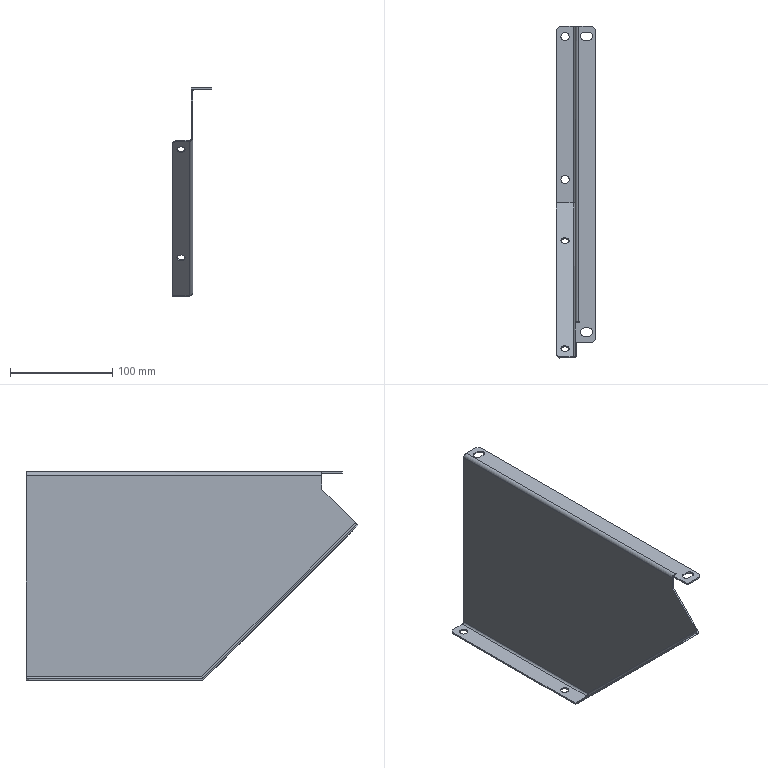Part | STEP file | SYL_0392D6J1SYL0380DJ100-138538 | 1 solid | 62 faces | box 38.5 x 325.355 x 203.95 mm | volume 94811 mm3 | plane 38 | spline 18 | cylinder 6 | commonest cylinder face diameters 4.1 x2 7 x2 4 x1 6.9 x1